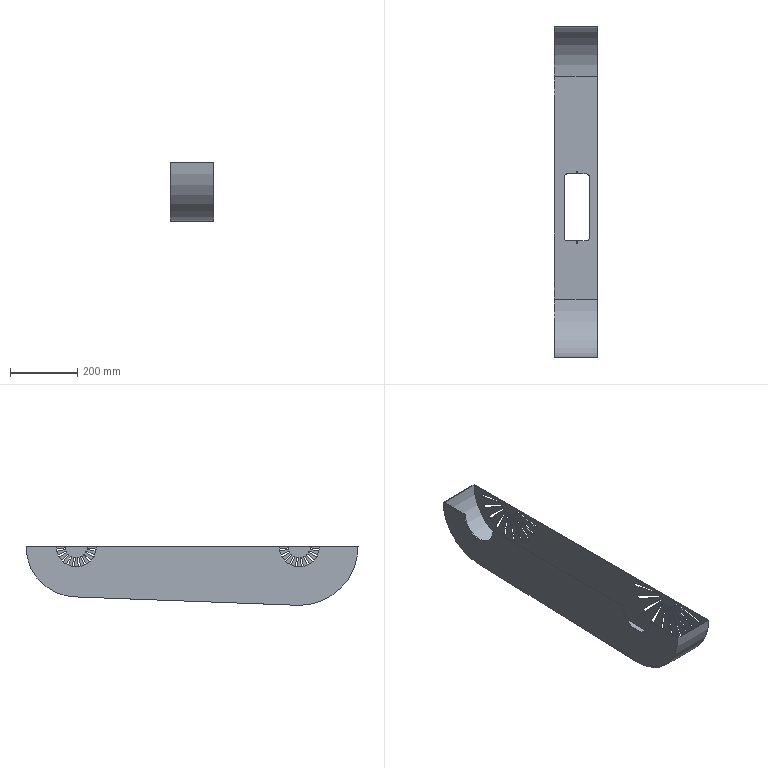Part | STEP file | Input 83 | 1 solid | 126 faces | box 130 x 990 x 175 mm | volume 933762 mm3 | cylinder 74 | plane 52 | commonest cylinder face diameters 5 x35 10 x29 20 x4 120 x2 295.4 x1 300 x1